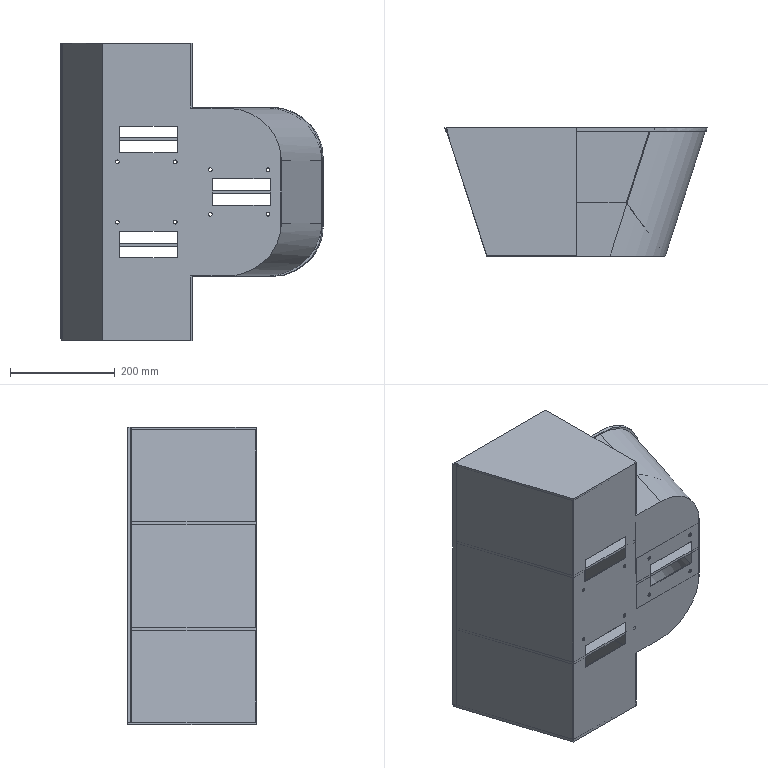Part | NX | features DATUM_CSYS 2, SKETCH 2, BREP 1, LINKED_FACE 1 | 1 solid | 102 faces | box 499.609 x 244.468 x 567.002 mm | volume 2802916 mm3 | plane 70 | cylinder 30 | spline 2 | commonest cylinder face diameters 7 x16 200 x6 1 x5 190 x2 4 x1